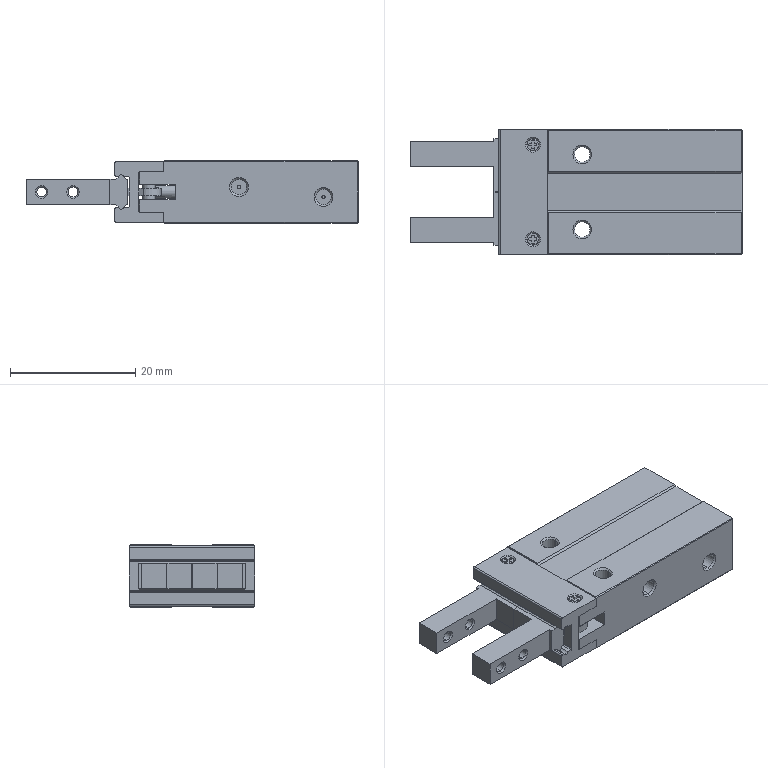Part | STEP file | HFZ6(CL)_HI | 1 solid | 342 faces | box 53 x 20 x 10 mm | volume 6778 mm3 | plane 174 | cylinder 122 | cone 46 | commonest cylinder face diameters 1 x21 1.3 x20 2 x18 2.459 x12 0.4 x10 1.567 x8